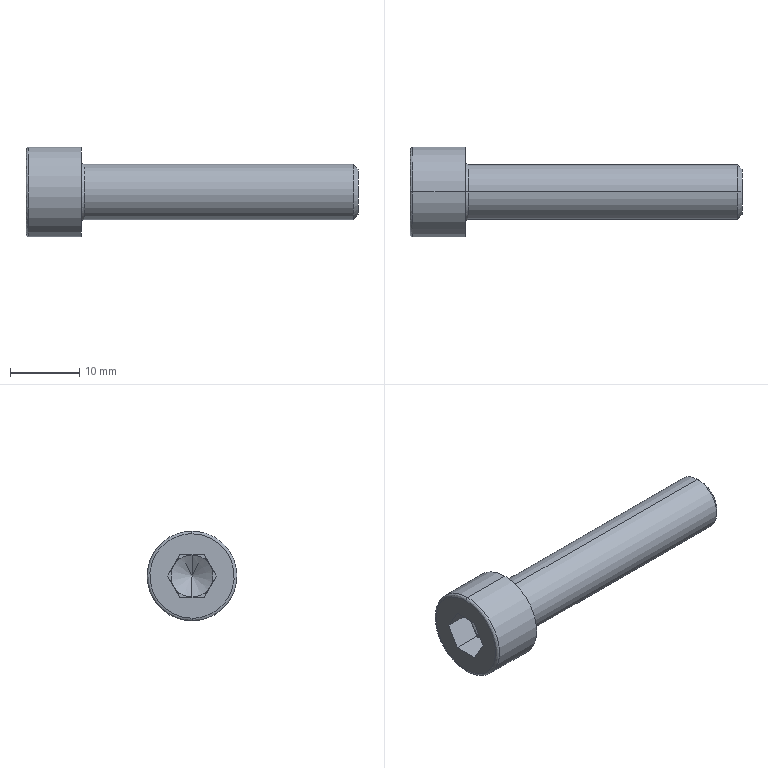Part | STEP file | PN_0007_default | 1 solid | 27 faces | box 48 x 13 x 13 mm | volume 2921 mm3 | plane 15 | spline 4 | cylinder 4 | cone 4 | commonest cylinder face diameters 8 x2 13 x2